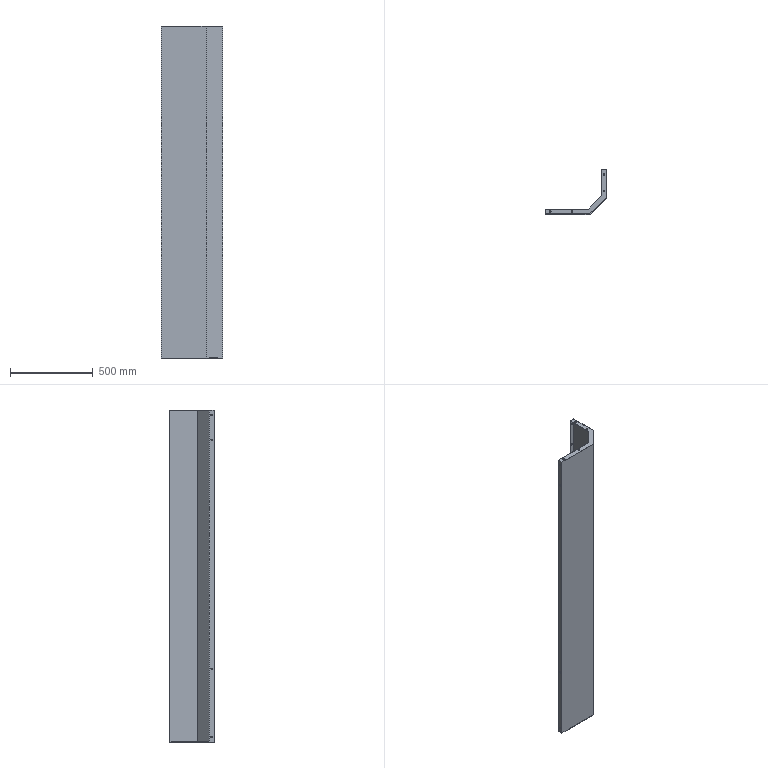Part | SolidWorks | features ICE 10, ExtruThin 1 | 1 solid | 48 faces | box 370 x 270 x 2005 mm | volume 2609209 mm3 | cylinder 30 | plane 18 | commonest cylinder face diameters 9 x30